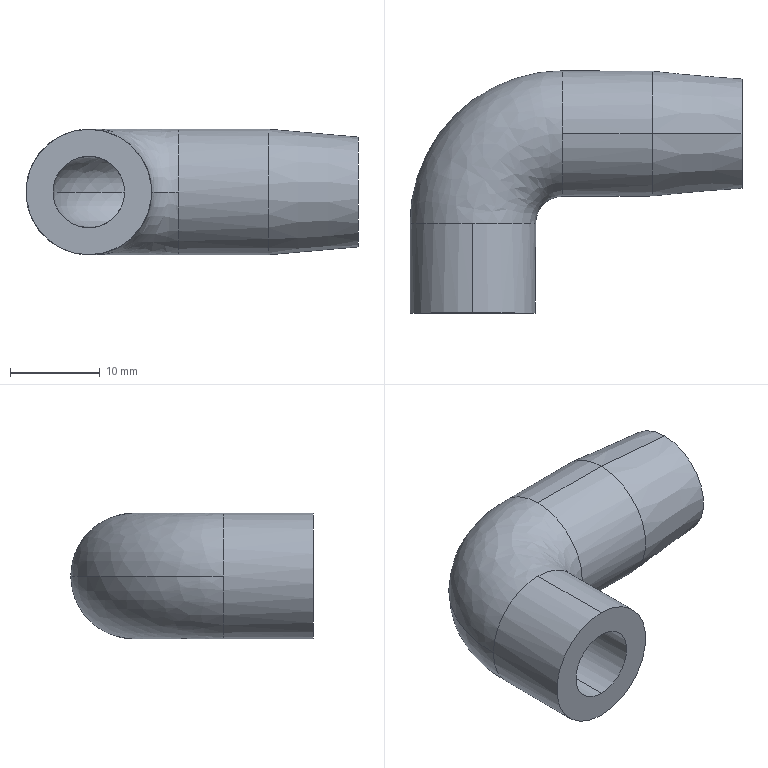Part | STEP file | noi khi | 1 solid | 18 faces | box 37 x 27 x 14 mm | volume 4436 mm3 | cylinder 8 | spline 4 | cone 4 | plane 2 | commonest cylinder face diameters 8 x4 14 x4